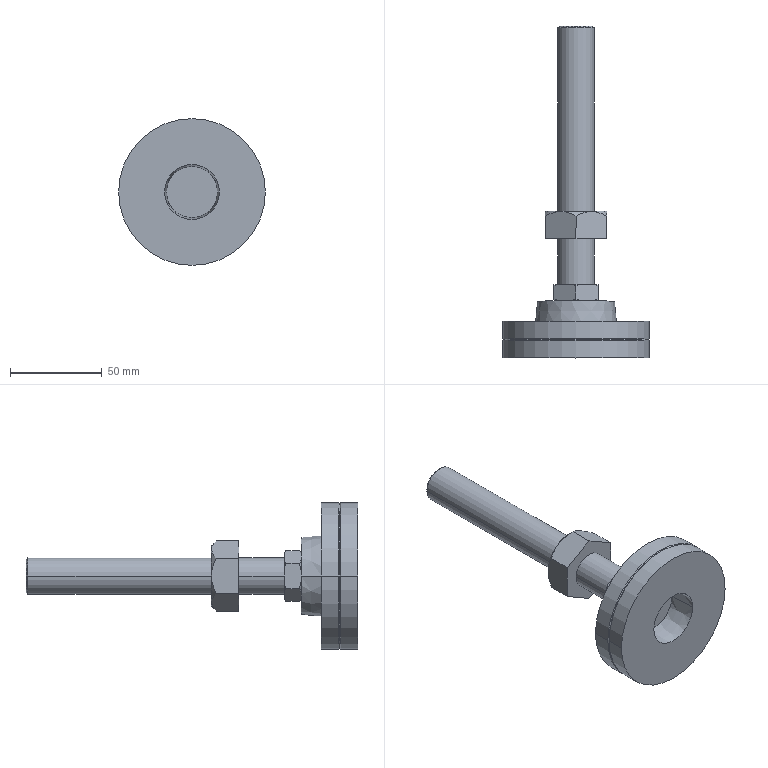Part | SolidWorks | features ICE 2, RevCut 2, Chamfer 1, Revolution 1 | 1 solid | 52 faces | box 80 x 181 x 80 mm | volume 164891 mm3 | cone 24 | plane 20 | cylinder 8 | commonest cylinder face diameters 20 x4 80 x4